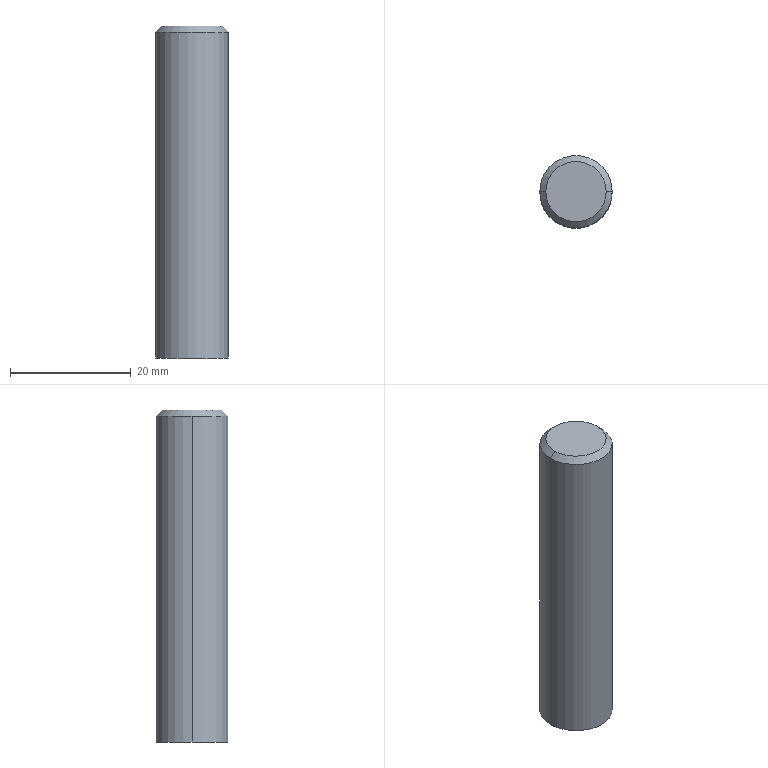Part | SolidWorks | features Chamfer 1, Extrusion 1 | 1 solid | 6 faces | box 12 x 12 x 55 mm | volume 6203 mm3 | cone 2 | cylinder 2 | plane 2 | commonest cylinder face diameters 12 x2
STEP:
#1=CARTESIAN_POINT('',(5.,0.,55.));
#2=VERTEX_POINT('',#1);
#3=CARTESIAN_POINT('',(-5.,0.,55.));
#4=VERTEX_POINT('',#3);
#5=CARTESIAN_POINT('',(0.,0.,55.));
#6=DIRECTION('',(0.,0.,1.));
#7=DIRECTION('',(1.,0.,0.));
#8=AXIS2_PLACEMENT_3D('',#5,#6,#7);
#9=CIRCLE('',#8,5.);
#10=EDGE_CURVE('',#2,#4,#9,.T.);
#11=ORIENTED_EDGE('',*,*,#10,.F.);
#12=CARTESIAN_POINT('',(6.,0.,54.));
#13=VERTEX_POINT('',#12);
#14=CARTESIAN_POINT('',(5.,0.,55.));
#15=DIRECTION('',(0.7071,0.,-0.7071));
#16=VECTOR('',#15,1000.);
#17=LINE('',#14,#16);
#18=EDGE_CURVE('',#2,#13,#17,.T.);
#19=ORIENTED_EDGE('',*,*,#18,.T.);
#20=CARTESIAN_POINT('',(-6.,0.,54.));
#21=VERTEX_POINT('',#20);
#22=CARTESIAN_POINT('',(0.,0.,54.));
#23=DIRECTION('',(0.,0.,-1.));
#24=DIRECTION('',(1.,0.,0.));
#25=AXIS2_PLACEMENT_3D('',#22,#23,#24);
#26=CIRCLE('',#25,6.);
#27=EDGE_CURVE('',#21,#13,#26,.T.);
#28=ORIENTED_EDGE('',*,*,#27,.F.);
#29=CARTESIAN_POINT('',(-5.,0.,55.));
#30=DIRECTION('',(-0.7071,0.,-0.7071));
#31=VECTOR('',#30,1000.);
#32=LINE('',#29,#31);
#33=EDGE_CURVE('',#4,#21,#32,.T.);
#34=ORIENTED_EDGE('',*,*,#33,.F.);
#35=EDGE_LOOP('',(#11,#19,#28,#34));
#36=FACE_OUTER_BOUND('',#35,.T.);
#37=CARTESIAN_POINT('',(0.,0.,55.));
#38=DIRECTION('',(0.,0.,-1.));
#39=DIRECTION('',(-1.,0.,0.));
#40=AXIS2_PLACEMENT_3D('',#37,#38,#39);
#41=CONICAL_SURFACE('',#40,5.,0.7854);
#42=ADVANCED_FACE('',(#36),#41,.T.);
#43=ORIENTED_EDGE('',*,*,#27,.T.);
#44=CARTESIAN_POINT('',(6.,0.,0.));
#45=VERTEX_POINT('',#44);
#46=CARTESIAN_POINT('',(6.,0.,55.));
#47=DIRECTION('',(0.,0.,-1.));
#48=VECTOR('',#47,1000.);
#49=LINE('',#46,#48);
#50=EDGE_CURVE('',#13,#45,#49,.T.);
#51=ORIENTED_EDGE('',*,*,#50,.T.);
#52=CARTESIAN_POINT('',(-6.,0.,0.));
#53=VERTEX_POINT('',#52);
#54=CARTESIAN_POINT('',(0.,0.,0.));
#55=DIRECTION('',(0.,0.,1.));
#56=DIRECTION('',(1.,0.,0.));
#57=AXIS2_PLACEMENT_3D('',#54,#55,#56);
#58=CIRCLE('',#57,6.);
#59=EDGE_CURVE('',#45,#53,#58,.T.);
#60=ORIENTED_EDGE('',*,*,#59,.T.);
#61=CARTESIAN_POINT('',(-6.,0.,55.));
#62=DIRECTION('',(0.,0.,-1.));
#63=VECTOR('',#62,1000.);
#64=LINE('',#61,#63);
#65=EDGE_CURVE('',#21,#53,#64,.T.);
#66=ORIENTED_EDGE('',*,*,#65,.F.);
#67=EDGE_LOOP('',(#43,#51,#60,#66));
#68=FACE_OUTER_BOUND('',#67,.T.);
#69=CARTESIAN_POINT('',(0.,0.,55.));
#70=DIRECTION('',(0.,0.,-1.));
#71=DIRECTION('',(-1.,0.,0.));
#72=AXIS2_PLACEMENT_3D('',#69,#70,#71);
#73=CYLINDRICAL_SURFACE('',#72,6.);
#74=ADVANCED_FACE('',(#68),#73,.T.);
#75=ORIENTED_EDGE('',*,*,#50,.F.);
#76=CARTESIAN_POINT('',(0.,0.,54.));
#77=DIRECTION('',(0.,0.,-1.));
#78=DIRECTION('',(1.,0.,0.));
#79=AXIS2_PLACEMENT_3D('',#76,#77,#78);
#80=CIRCLE('',#79,6.);
#81=EDGE_CURVE('',#13,#21,#80,.T.);
#82=ORIENTED_EDGE('',*,*,#81,.T.);
#83=ORIENTED_EDGE('',*,*,#65,.T.);
#84=CARTESIAN_POINT('',(0.,0.,0.));
#85=DIRECTION('',(0.,0.,1.));
#86=DIRECTION('',(1.,0.,0.));
#87=AXIS2_PLACEMENT_3D('',#84,#85,#86);
#88=CIRCLE('',#87,6.);
#89=EDGE_CURVE('',#53,#45,#88,.T.);
#90=ORIENTED_EDGE('',*,*,#89,.T.);
#91=EDGE_LOOP('',(#75,#82,#83,#90));
#92=FACE_OUTER_BOUND('',#91,.T.);
#93=CARTESIAN_POINT('',(0.,0.,55.));
#94=DIRECTION('',(0.,0.,-1.));
#95=DIRECTION('',(-1.,0.,0.));
#96=AXIS2_PLACEMENT_3D('',#93,#94,#95);
#97=CYLINDRICAL_SURFACE('',#96,6.);
#98=ADVANCED_FACE('',(#92),#97,.T.);
#99=CARTESIAN_POINT('',(0.,0.,55.));
#100=DIRECTION('',(0.,0.,1.));
#101=DIRECTION('',(1.,0.,0.));
#102=AXIS2_PLACEMENT_3D('',#99,#100,#101);
#103=CIRCLE('',#102,5.);
#104=EDGE_CURVE('',#4,#2,#103,.T.);
#105=ORIENTED_EDGE('',*,*,#104,.T.);
#106=ORIENTED_EDGE('',*,*,#10,.T.);
#107=EDGE_LOOP('',(#105,#106));
#108=FACE_OUTER_BOUND('',#107,.T.);
#109=CARTESIAN_POINT('',(0.,0.,55.));
#110=DIRECTION('',(0.,0.,1.));
#111=DIRECTION('',(1.,0.,0.));
#112=AXIS2_PLACEMENT_3D('',#109,#110,#111);
#113=PLANE('',#112);
#114=ADVANCED_FACE('',(#108),#113,.T.);
#115=ORIENTED_EDGE('',*,*,#89,.F.);
#116=ORIENTED_EDGE('',*,*,#59,.F.);
#117=EDGE_LOOP('',(#115,#116));
#118=FACE_OUTER_BOUND('',#117,.T.);
#119=CARTESIAN_POINT('',(0.,0.,0.));
#120=DIRECTION('',(0.,0.,1.));
#121=DIRECTION('',(1.,0.,0.));
#122=AXIS2_PLACEMENT_3D('',#119,#120,#121);
#123=PLANE('',#122);
#124=ADVANCED_FACE('',(#118),#123,.F.);
#125=ORIENTED_EDGE('',*,*,#18,.F.);
#126=ORIENTED_EDGE('',*,*,#104,.F.);
#127=ORIENTED_EDGE('',*,*,#33,.T.);
#128=ORIENTED_EDGE('',*,*,#81,.F.);
#129=EDGE_LOOP('',(#125,#126,#127,#128));
#130=FACE_OUTER_BOUND('',#129,.T.);
#131=CARTESIAN_POINT('',(0.,0.,55.));
#132=DIRECTION('',(0.,0.,-1.));
#133=DIRECTION('',(-1.,0.,0.));
#134=AXIS2_PLACEMENT_3D('',#131,#132,#133);
#135=CONICAL_SURFACE('',#134,5.,0.7854);
#136=ADVANCED_FACE('',(#130),#135,.T.);
#137=CLOSED_SHELL('',(#42,#74,#98,#114,#124,#136));
#138=MANIFOLD_SOLID_BREP('',#137);
#139=CARTESIAN_POINT('',(0.,0.,0.));
#140=DIRECTION('',(0.,0.,1.));
#141=DIRECTION('',(1.,0.,0.));
#142=AXIS2_PLACEMENT_3D('',#139,#140,#141);
#143=(LENGTH_UNIT()NAMED_UNIT(*)SI_UNIT(.MILLI.,.METRE.));
#144=UNCERTAINTY_MEASURE_WITH_UNIT(LENGTH_MEASURE(0.00001),#143,'','');
#145=(NAMED_UNIT(*)PLANE_ANGLE_UNIT()SI_UNIT($,.RADIAN.));
#146=(NAMED_UNIT(*)SI_UNIT($,.STERADIAN.)SOLID_ANGLE_UNIT());
#147=(GEOMETRIC_REPRESENTATION_CONTEXT(3)GLOBAL_UNCERTAINTY_ASSIGNED_CONTEXT((#144))GLOBAL_UNIT_ASSIGNED_CONTEXT((#143,#145,#146))REPRESENTATION_CONTEXT('',''));
#148=ADVANCED_BREP_SHAPE_REPRESENTATION('',(#138,#142),#147);